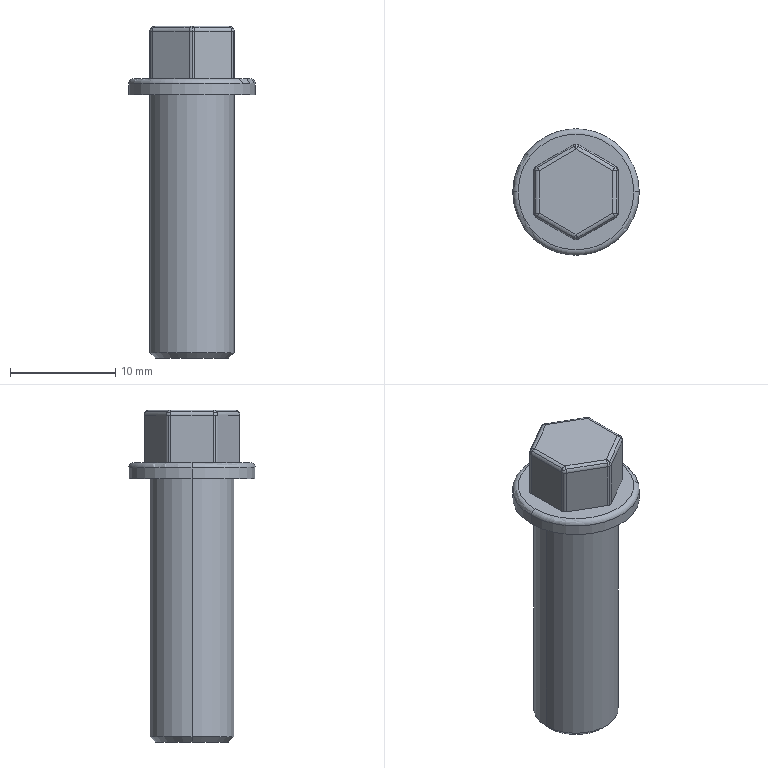Part | SolidWorks | features BaseBody 1 | 1 solid | 54 faces | box 12 x 12 x 31.5 mm | volume 1697 mm3 | cylinder 28 | sphere 12 | plane 10 | torus 2 | cone 2 | commonest cylinder face diameters 1 x24 8 x2 12 x2
STEP:
#1=CARTESIAN_POINT('',(-3.947,2.021,6.224));
#2=VERTEX_POINT('',#1);
#3=CARTESIAN_POINT('',(-4.,2.021,6.));
#4=VERTEX_POINT('',#3);
#5=CARTESIAN_POINT('',(-3.5,2.021,6.));
#6=DIRECTION('',(0.,-1.,0.));
#7=DIRECTION('',(0.,0.,1.));
#8=AXIS2_PLACEMENT_3D('',#5,#6,#7);
#9=CIRCLE('',#8,0.5);
#10=EDGE_CURVE('',#2,#4,#9,.T.);
#11=ORIENTED_EDGE('',*,*,#10,.F.);
#12=CARTESIAN_POINT('',(-3.724,2.408,6.224));
#13=VERTEX_POINT('',#12);
#14=CARTESIAN_POINT('',(-3.5,2.021,6.));
#15=DIRECTION('',(-0.433,0.25,-0.866));
#16=DIRECTION('',(-0.8944,0.,0.4472));
#17=AXIS2_PLACEMENT_3D('',#14,#15,#16);
#18=CIRCLE('',#17,0.5);
#19=EDGE_CURVE('',#2,#13,#18,.T.);
#20=ORIENTED_EDGE('',*,*,#19,.T.);
#21=CARTESIAN_POINT('',(-3.75,2.454,6.));
#22=VERTEX_POINT('',#21);
#23=CARTESIAN_POINT('',(-3.5,2.021,6.));
#24=DIRECTION('',(0.866,0.5,0.));
#25=DIRECTION('',(-0.5,0.866,0.));
#26=AXIS2_PLACEMENT_3D('',#23,#24,#25);
#27=CIRCLE('',#26,0.5);
#28=EDGE_CURVE('',#22,#13,#27,.T.);
#29=ORIENTED_EDGE('',*,*,#28,.F.);
#30=CARTESIAN_POINT('',(-3.933,2.271,6.));
#31=VERTEX_POINT('',#30);
#32=CARTESIAN_POINT('',(-3.5,2.021,6.));
#33=DIRECTION('',(0.,0.,-1.));
#34=DIRECTION('',(-1.,0.,0.));
#35=AXIS2_PLACEMENT_3D('',#32,#33,#34);
#36=CIRCLE('',#35,0.5);
#37=EDGE_CURVE('',#31,#22,#36,.T.);
#38=ORIENTED_EDGE('',*,*,#37,.F.);
#39=CARTESIAN_POINT('',(-3.5,2.021,6.));
#40=DIRECTION('',(0.,0.,-1.));
#41=DIRECTION('',(-1.,0.,0.));
#42=AXIS2_PLACEMENT_3D('',#39,#40,#41);
#43=CIRCLE('',#42,0.5);
#44=EDGE_CURVE('',#4,#31,#43,.T.);
#45=ORIENTED_EDGE('',*,*,#44,.F.);
#46=EDGE_LOOP('',(#11,#20,#29,#38,#45));
#47=FACE_OUTER_BOUND('',#46,.T.);
#48=CARTESIAN_POINT('',(-3.5,2.021,6.));
#49=DIRECTION('',(0.433,-0.25,0.866));
#50=DIRECTION('',(-0.75,0.433,0.5));
#51=AXIS2_PLACEMENT_3D('',#48,#49,#50);
#52=SPHERICAL_SURFACE('',#51,0.5);
#53=ADVANCED_FACE('',(#47),#52,.T.);
#54=ORIENTED_EDGE('',*,*,#44,.T.);
#55=CARTESIAN_POINT('',(-3.933,2.271,1.5));
#56=VERTEX_POINT('',#55);
#57=CARTESIAN_POINT('',(-3.933,2.271,1.5));
#58=DIRECTION('',(0.,0.,-1.));
#59=VECTOR('',#58,1000.);
#60=LINE('',#57,#59);
#61=EDGE_CURVE('',#31,#56,#60,.T.);
#62=ORIENTED_EDGE('',*,*,#61,.T.);
#63=CARTESIAN_POINT('',(-4.,2.021,1.5));
#64=VERTEX_POINT('',#63);
#65=CARTESIAN_POINT('',(-3.5,2.021,1.5));
#66=DIRECTION('',(0.,0.,1.));
#67=DIRECTION('',(-0.866,0.5,0.));
#68=AXIS2_PLACEMENT_3D('',#65,#66,#67);
#69=CIRCLE('',#68,0.5);
#70=EDGE_CURVE('',#56,#64,#69,.T.);
#71=ORIENTED_EDGE('',*,*,#70,.T.);
#72=CARTESIAN_POINT('',(-4.,2.021,1.5));
#73=DIRECTION('',(0.,0.,1.));
#74=VECTOR('',#73,1000.);
#75=LINE('',#72,#74);
#76=EDGE_CURVE('',#64,#4,#75,.T.);
#77=ORIENTED_EDGE('',*,*,#76,.T.);
#78=EDGE_LOOP('',(#54,#62,#71,#77));
#79=FACE_OUTER_BOUND('',#78,.T.);
#80=CARTESIAN_POINT('',(-3.5,2.021,1.5));
#81=DIRECTION('',(0.,0.,-1.));
#82=DIRECTION('',(-0.866,0.5,0.));
#83=AXIS2_PLACEMENT_3D('',#80,#81,#82);
#84=CYLINDRICAL_SURFACE('',#83,0.5);
#85=ADVANCED_FACE('',(#79),#84,.T.);
#86=CARTESIAN_POINT('',(-3.724,-2.408,6.224));
#87=VERTEX_POINT('',#86);
#88=CARTESIAN_POINT('',(-3.75,-2.454,6.));
#89=VERTEX_POINT('',#88);
#90=CARTESIAN_POINT('',(-3.5,-2.021,6.));
#91=DIRECTION('',(0.866,-0.5,0.));
#92=DIRECTION('',(0.,0.,1.));
#93=AXIS2_PLACEMENT_3D('',#90,#91,#92);
#94=CIRCLE('',#93,0.5);
#95=EDGE_CURVE('',#87,#89,#94,.T.);
#96=ORIENTED_EDGE('',*,*,#95,.F.);
#97=CARTESIAN_POINT('',(-3.947,-2.021,6.224));
#98=VERTEX_POINT('',#97);
#99=CARTESIAN_POINT('',(-3.5,-2.021,6.));
#100=DIRECTION('',(-0.433,-0.25,-0.866));
#101=DIRECTION('',(-0.8944,0.,0.4472));
#102=AXIS2_PLACEMENT_3D('',#99,#100,#101);
#103=CIRCLE('',#102,0.5);
#104=EDGE_CURVE('',#87,#98,#103,.T.);
#105=ORIENTED_EDGE('',*,*,#104,.T.);
#106=CARTESIAN_POINT('',(-4.,-2.021,6.));
#107=VERTEX_POINT('',#106);
#108=CARTESIAN_POINT('',(-3.5,-2.021,6.));
#109=DIRECTION('',(0.,1.,0.));
#110=DIRECTION('',(-1.,0.,0.));
#111=AXIS2_PLACEMENT_3D('',#108,#109,#110);
#112=CIRCLE('',#111,0.5);
#113=EDGE_CURVE('',#107,#98,#112,.T.);
#114=ORIENTED_EDGE('',*,*,#113,.F.);
#115=CARTESIAN_POINT('',(-3.933,-2.271,6.));
#116=VERTEX_POINT('',#115);
#117=CARTESIAN_POINT('',(-3.5,-2.021,6.));
#118=DIRECTION('',(0.,0.,-1.));
#119=DIRECTION('',(-0.5,-0.866,0.));
#120=AXIS2_PLACEMENT_3D('',#117,#118,#119);
#121=CIRCLE('',#120,0.5);
#122=EDGE_CURVE('',#116,#107,#121,.T.);
#123=ORIENTED_EDGE('',*,*,#122,.F.);
#124=CARTESIAN_POINT('',(-3.5,-2.021,6.));
#125=DIRECTION('',(0.,0.,-1.));
#126=DIRECTION('',(-0.5,-0.866,0.));
#127=AXIS2_PLACEMENT_3D('',#124,#125,#126);
#128=CIRCLE('',#127,0.5);
#129=EDGE_CURVE('',#89,#116,#128,.T.);
#130=ORIENTED_EDGE('',*,*,#129,.F.);
#131=EDGE_LOOP('',(#96,#105,#114,#123,#130));
#132=FACE_OUTER_BOUND('',#131,.T.);
#133=CARTESIAN_POINT('',(-3.5,-2.021,6.));
#134=DIRECTION('',(0.433,0.25,0.866));
#135=DIRECTION('',(-0.75,-0.433,0.5));
#136=AXIS2_PLACEMENT_3D('',#133,#134,#135);
#137=SPHERICAL_SURFACE('',#136,0.5);
#138=ADVANCED_FACE('',(#132),#137,.T.);
#139=ORIENTED_EDGE('',*,*,#129,.T.);
#140=CARTESIAN_POINT('',(-3.933,-2.271,1.5));
#141=VERTEX_POINT('',#140);
#142=CARTESIAN_POINT('',(-3.933,-2.271,1.5));
#143=DIRECTION('',(0.,0.,-1.));
#144=VECTOR('',#143,1000.);
#145=LINE('',#142,#144);
#146=EDGE_CURVE('',#116,#141,#145,.T.);
#147=ORIENTED_EDGE('',*,*,#146,.T.);
#148=CARTESIAN_POINT('',(-3.75,-2.454,1.5));
#149=VERTEX_POINT('',#148);
#150=CARTESIAN_POINT('',(-3.5,-2.021,1.5));
#151=DIRECTION('',(0.,0.,1.));
#152=DIRECTION('',(-0.866,-0.5,0.));
#153=AXIS2_PLACEMENT_3D('',#150,#151,#152);
#154=CIRCLE('',#153,0.5);
#155=EDGE_CURVE('',#141,#149,#154,.T.);
#156=ORIENTED_EDGE('',*,*,#155,.T.);
#157=CARTESIAN_POINT('',(-3.75,-2.454,1.5));
#158=DIRECTION('',(0.,0.,1.));
#159=VECTOR('',#158,1000.);
#160=LINE('',#157,#159);
#161=EDGE_CURVE('',#149,#89,#160,.T.);
#162=ORIENTED_EDGE('',*,*,#161,.T.);
#163=EDGE_LOOP('',(#139,#147,#156,#162));
#164=FACE_OUTER_BOUND('',#163,.T.);
#165=CARTESIAN_POINT('',(-3.5,-2.021,1.5));
#166=DIRECTION('',(0.,0.,-1.));
#167=DIRECTION('',(-0.866,-0.5,0.));
#168=AXIS2_PLACEMENT_3D('',#165,#166,#167);
#169=CYLINDRICAL_SURFACE('',#168,0.5);
#170=ADVANCED_FACE('',(#164),#169,.T.);
#171=CARTESIAN_POINT('',(0.,4.041,6.5));
#172=VERTEX_POINT('',#171);
#173=CARTESIAN_POINT('',(-0.1768,4.348,6.354));
#174=VERTEX_POINT('',#173);
#175=CARTESIAN_POINT('',(0.,4.041,6.));
#176=DIRECTION('',(-0.866,-0.5,0.));
#177=DIRECTION('',(0.,0.,1.));
#178=AXIS2_PLACEMENT_3D('',#175,#176,#177);
#179=CIRCLE('',#178,0.5);
#180=EDGE_CURVE('',#172,#174,#179,.T.);
#181=ORIENTED_EDGE('',*,*,#180,.F.);
#182=CARTESIAN_POINT('',(0.,4.541,6.));
#183=VERTEX_POINT('',#182);
#184=CARTESIAN_POINT('',(0.,4.041,6.));
#185=DIRECTION('',(-1.,0.,0.));
#186=DIRECTION('',(0.,-1.,0.));
#187=AXIS2_PLACEMENT_3D('',#184,#185,#186);
#188=CIRCLE('',#187,0.5);
#189=EDGE_CURVE('',#172,#183,#188,.T.);
#190=ORIENTED_EDGE('',*,*,#189,.T.);
#191=CARTESIAN_POINT('',(-0.25,4.474,6.));
#192=VERTEX_POINT('',#191);
#193=CARTESIAN_POINT('',(0.,4.041,6.));
#194=DIRECTION('',(0.,0.,-1.));
#195=DIRECTION('',(-0.5,0.866,0.));
#196=AXIS2_PLACEMENT_3D('',#193,#194,#195);
#197=CIRCLE('',#196,0.5);
#198=EDGE_CURVE('',#192,#183,#197,.T.);
#199=ORIENTED_EDGE('',*,*,#198,.F.);
#200=CARTESIAN_POINT('',(0.,4.041,6.));
#201=DIRECTION('',(-0.866,-0.5,0.));
#202=DIRECTION('',(0.,0.,1.));
#203=AXIS2_PLACEMENT_3D('',#200,#201,#202);
#204=CIRCLE('',#203,0.5);
#205=EDGE_CURVE('',#174,#192,#204,.T.);
#206=ORIENTED_EDGE('',*,*,#205,.F.);
#207=EDGE_LOOP('',(#181,#190,#199,#206));
#208=FACE_OUTER_BOUND('',#207,.T.);
#209=CARTESIAN_POINT('',(0.,4.041,6.));
#210=DIRECTION('',(1.,0.,0.));
#211=DIRECTION('',(0.,0.866,0.5));
#212=AXIS2_PLACEMENT_3D('',#209,#210,#211);
#213=SPHERICAL_SURFACE('',#212,0.5);
#214=ADVANCED_FACE('',(#208),#213,.T.);
#215=ORIENTED_EDGE('',*,*,#198,.T.);
#216=CARTESIAN_POINT('',(0.,4.541,1.5));
#217=VERTEX_POINT('',#216);
#218=CARTESIAN_POINT('',(0.,4.541,1.5));
#219=DIRECTION('',(0.,0.,-1.));
#220=VECTOR('',#219,1000.);
#221=LINE('',#218,#220);
#222=EDGE_CURVE('',#183,#217,#221,.T.);
#223=ORIENTED_EDGE('',*,*,#222,.T.);
#224=CARTESIAN_POINT('',(-0.25,4.474,1.5));
#225=VERTEX_POINT('',#224);
#226=CARTESIAN_POINT('',(0.,4.041,1.5));
#227=DIRECTION('',(0.,0.,1.));
#228=DIRECTION('',(0.,1.,0.));
#229=AXIS2_PLACEMENT_3D('',#226,#227,#228);
#230=CIRCLE('',#229,0.5);
#231=EDGE_CURVE('',#217,#225,#230,.T.);
#232=ORIENTED_EDGE('',*,*,#231,.T.);
#233=CARTESIAN_POINT('',(-0.25,4.474,1.5));
#234=DIRECTION('',(0.,0.,1.));
#235=VECTOR('',#234,1000.);
#236=LINE('',#233,#235);
#237=EDGE_CURVE('',#225,#192,#236,.T.);
#238=ORIENTED_EDGE('',*,*,#237,.T.);
#239=EDGE_LOOP('',(#215,#223,#232,#238));
#240=FACE_OUTER_BOUND('',#239,.T.);
#241=CARTESIAN_POINT('',(0.,4.041,1.5));
#242=DIRECTION('',(0.,0.,-1.));
#243=DIRECTION('',(0.,1.,0.));
#244=AXIS2_PLACEMENT_3D('',#241,#242,#243);
#245=CYLINDRICAL_SURFACE('',#244,0.5);
#246=ADVANCED_FACE('',(#240),#245,.T.);
#247=ORIENTED_EDGE('',*,*,#28,.T.);
#248=CARTESIAN_POINT('',(-3.677,2.327,6.354));
#249=VERTEX_POINT('',#248);
#250=CARTESIAN_POINT('',(-3.5,2.021,6.));
#251=DIRECTION('',(0.866,0.5,0.));
#252=DIRECTION('',(-0.5,0.866,0.));
#253=AXIS2_PLACEMENT_3D('',#250,#251,#252);
#254=CIRCLE('',#253,0.5);
#255=EDGE_CURVE('',#13,#249,#254,.T.);
#256=ORIENTED_EDGE('',*,*,#255,.T.);
#257=CARTESIAN_POINT('',(-0.9268,3.915,6.354));
#258=DIRECTION('',(0.866,0.5,0.));
#259=VECTOR('',#258,1000.);
#260=LINE('',#257,#259);
#261=EDGE_CURVE('',#249,#174,#260,.T.);
#262=ORIENTED_EDGE('',*,*,#261,.T.);
#263=ORIENTED_EDGE('',*,*,#205,.T.);
#264=CARTESIAN_POINT('',(-1.,4.041,6.));
#265=DIRECTION('',(-0.866,-0.5,0.));
#266=VECTOR('',#265,1000.);
#267=LINE('',#264,#266);
#268=EDGE_CURVE('',#192,#22,#267,.T.);
#269=ORIENTED_EDGE('',*,*,#268,.T.);
#270=EDGE_LOOP('',(#247,#256,#262,#263,#269));
#271=FACE_OUTER_BOUND('',#270,.T.);
#272=CARTESIAN_POINT('',(-0.75,3.608,6.));
#273=DIRECTION('',(0.866,0.5,0.));
#274=DIRECTION('',(-0.3536,0.6124,0.7071));
#275=AXIS2_PLACEMENT_3D('',#272,#273,#274);
#276=CYLINDRICAL_SURFACE('',#275,0.5);
#277=ADVANCED_FACE('',(#271),#276,.T.);
#278=CARTESIAN_POINT('',(0.,-4.541,6.));
#279=VERTEX_POINT('',#278);
#280=CARTESIAN_POINT('',(-0.25,-4.474,6.));
#281=VERTEX_POINT('',#280);
#282=CARTESIAN_POINT('',(0.,-4.041,6.));
#283=DIRECTION('',(0.,0.,-1.));
#284=DIRECTION('',(0.5,-0.866,0.));
#285=AXIS2_PLACEMENT_3D('',#282,#283,#284);
#286=CIRCLE('',#285,0.5);
#287=EDGE_CURVE('',#279,#281,#286,.T.);
#288=ORIENTED_EDGE('',*,*,#287,.F.);
#289=CARTESIAN_POINT('',(0.,-4.041,6.5));
#290=VERTEX_POINT('',#289);
#291=CARTESIAN_POINT('',(0.,-4.041,6.));
#292=DIRECTION('',(-1.,0.,0.));
#293=DIRECTION('',(0.,-1.,0.));
#294=AXIS2_PLACEMENT_3D('',#291,#292,#293);
#295=CIRCLE('',#294,0.5);
#296=EDGE_CURVE('',#279,#290,#295,.T.);
#297=ORIENTED_EDGE('',*,*,#296,.T.);
#298=CARTESIAN_POINT('',(-0.1768,-4.348,6.354));
#299=VERTEX_POINT('',#298);
#300=CARTESIAN_POINT('',(0.,-4.041,6.));
#301=DIRECTION('',(-0.866,0.5,0.));
#302=DIRECTION('',(-0.5,-0.866,0.));
#303=AXIS2_PLACEMENT_3D('',#300,#301,#302);
#304=CIRCLE('',#303,0.5);
#305=EDGE_CURVE('',#299,#290,#304,.T.);
#306=ORIENTED_EDGE('',*,*,#305,.F.);
#307=CARTESIAN_POINT('',(0.,-4.041,6.));
#308=DIRECTION('',(-0.866,0.5,0.));
#309=DIRECTION('',(-0.5,-0.866,0.));
#310=AXIS2_PLACEMENT_3D('',#307,#308,#309);
#311=CIRCLE('',#310,0.5);
#312=EDGE_CURVE('',#281,#299,#311,.T.);
#313=ORIENTED_EDGE('',*,*,#312,.F.);
#314=EDGE_LOOP('',(#288,#297,#306,#313));
#315=FACE_OUTER_BOUND('',#314,.T.);
#316=CARTESIAN_POINT('',(0.,-4.041,6.));
#317=DIRECTION('',(1.,0.,0.));
#318=DIRECTION('',(0.,-0.866,0.5));
#319=AXIS2_PLACEMENT_3D('',#316,#317,#318);
#320=SPHERICAL_SURFACE('',#319,0.5);
#321=ADVANCED_FACE('',(#315),#320,.T.);
#322=CARTESIAN_POINT('',(0.25,-4.474,6.));
#323=VERTEX_POINT('',#322);
#324=CARTESIAN_POINT('',(0.,-4.041,6.));
#325=DIRECTION('',(0.,0.,-1.));
#326=DIRECTION('',(0.5,-0.866,0.));
#327=AXIS2_PLACEMENT_3D('',#324,#325,#326);
#328=CIRCLE('',#327,0.5);
#329=EDGE_CURVE('',#323,#279,#328,.T.);
#330=ORIENTED_EDGE('',*,*,#329,.T.);
#331=CARTESIAN_POINT('',(0.,-4.541,1.5));
#332=VERTEX_POINT('',#331);
#333=CARTESIAN_POINT('',(0.,-4.541,1.5));
#334=DIRECTION('',(0.,0.,-1.));
#335=VECTOR('',#334,1000.);
#336=LINE('',#333,#335);
#337=EDGE_CURVE('',#279,#332,#336,.T.);
#338=ORIENTED_EDGE('',*,*,#337,.T.);
#339=CARTESIAN_POINT('',(0.25,-4.474,1.5));
#340=VERTEX_POINT('',#339);
#341=CARTESIAN_POINT('',(0.,-4.041,1.5));
#342=DIRECTION('',(0.,0.,1.));
#343=DIRECTION('',(0.,-1.,0.));
#344=AXIS2_PLACEMENT_3D('',#341,#342,#343);
#345=CIRCLE('',#344,0.5);
#346=EDGE_CURVE('',#332,#340,#345,.T.);
#347=ORIENTED_EDGE('',*,*,#346,.T.);
#348=CARTESIAN_POINT('',(0.25,-4.474,1.5));
#349=DIRECTION('',(0.,0.,1.));
#350=VECTOR('',#349,1000.);
#351=LINE('',#348,#350);
#352=EDGE_CURVE('',#340,#323,#351,.T.);
#353=ORIENTED_EDGE('',*,*,#352,.T.);
#354=EDGE_LOOP('',(#330,#338,#347,#353));
#355=FACE_OUTER_BOUND('',#354,.T.);
#356=CARTESIAN_POINT('',(0.,-4.041,1.5));
#357=DIRECTION('',(0.,0.,-1.));
#358=DIRECTION('',(0.,-1.,0.));
#359=AXIS2_PLACEMENT_3D('',#356,#357,#358);
#360=CYLINDRICAL_SURFACE('',#359,0.5);
#361=ADVANCED_FACE('',(#355),#360,.T.);
#362=CARTESIAN_POINT('',(3.724,2.408,6.224));
#363=VERTEX_POINT('',#362);
#364=CARTESIAN_POINT('',(3.75,2.454,6.));
#365=VERTEX_POINT('',#364);
#366=CARTESIAN_POINT('',(3.5,2.021,6.));
#367=DIRECTION('',(-0.866,0.5,0.));
#368=DIRECTION('',(0.,0.,1.));
#369=AXIS2_PLACEMENT_3D('',#366,#367,#368);
#370=CIRCLE('',#369,0.5);
#371=EDGE_CURVE('',#363,#365,#370,.T.);
#372=ORIENTED_EDGE('',*,*,#371,.F.);
#373=CARTESIAN_POINT('',(3.947,2.021,6.224));
#374=VERTEX_POINT('',#373);
#375=CARTESIAN_POINT('',(3.5,2.021,6.));
#376=DIRECTION('',(0.433,0.25,-0.866));
#377=DIRECTION('',(-0.8944,0.,-0.4472));
#378=AXIS2_PLACEMENT_3D('',#375,#376,#377);
#379=CIRCLE('',#378,0.5);
#380=EDGE_CURVE('',#363,#374,#379,.T.);
#381=ORIENTED_EDGE('',*,*,#380,.T.);
#382=CARTESIAN_POINT('',(4.,2.021,6.));
#383=VERTEX_POINT('',#382);
#384=CARTESIAN_POINT('',(3.5,2.021,6.));
#385=DIRECTION('',(0.,-1.,0.));
#386=DIRECTION('',(1.,0.,0.));
#387=AXIS2_PLACEMENT_3D('',#384,#385,#386);
#388=CIRCLE('',#387,0.5);
#389=EDGE_CURVE('',#383,#374,#388,.T.);
#390=ORIENTED_EDGE('',*,*,#389,.F.);
#391=CARTESIAN_POINT('',(3.933,2.271,6.));
#392=VERTEX_POINT('',#391);
#393=CARTESIAN_POINT('',(3.5,2.021,6.));
#394=DIRECTION('',(0.,0.,-1.));
#395=DIRECTION('',(0.5,0.866,0.));
#396=AXIS2_PLACEMENT_3D('',#393,#394,#395);
#397=CIRCLE('',#396,0.5);
#398=EDGE_CURVE('',#392,#383,#397,.T.);
#399=ORIENTED_EDGE('',*,*,#398,.F.);
#400=CARTESIAN_POINT('',(3.5,2.021,6.));
#401=DIRECTION('',(0.,0.,-1.));
#402=DIRECTION('',(0.5,0.866,0.));
#403=AXIS2_PLACEMENT_3D('',#400,#401,#402);
#404=CIRCLE('',#403,0.5);
#405=EDGE_CURVE('',#365,#392,#404,.T.);
#406=ORIENTED_EDGE('',*,*,#405,.F.);
#407=EDGE_LOOP('',(#372,#381,#390,#399,#406));
#408=FACE_OUTER_BOUND('',#407,.T.);
#409=CARTESIAN_POINT('',(3.5,2.021,6.));
#410=DIRECTION('',(-0.433,-0.25,0.866));
#411=DIRECTION('',(0.75,0.433,0.5));
#412=AXIS2_PLACEMENT_3D('',#409,#410,#411);
#413=SPHERICAL_SURFACE('',#412,0.5);
#414=ADVANCED_FACE('',(#408),#413,.T.);
#415=ORIENTED_EDGE('',*,*,#405,.T.);
#416=CARTESIAN_POINT('',(3.933,2.271,1.5));
#417=VERTEX_POINT('',#416);
#418=CARTESIAN_POINT('',(3.933,2.271,1.5));
#419=DIRECTION('',(0.,0.,-1.));
#420=VECTOR('',#419,1000.);
#421=LINE('',#418,#420);
#422=EDGE_CURVE('',#392,#417,#421,.T.);
#423=ORIENTED_EDGE('',*,*,#422,.T.);
#424=CARTESIAN_POINT('',(3.75,2.454,1.5));
#425=VERTEX_POINT('',#424);
#426=CARTESIAN_POINT('',(3.5,2.021,1.5));
#427=DIRECTION('',(0.,0.,1.));
#428=DIRECTION('',(0.866,0.5,0.));
#429=AXIS2_PLACEMENT_3D('',#426,#427,#428);
#430=CIRCLE('',#429,0.5);
#431=EDGE_CURVE('',#417,#425,#430,.T.);
#432=ORIENTED_EDGE('',*,*,#431,.T.);
#433=CARTESIAN_POINT('',(3.75,2.454,1.5));
#434=DIRECTION('',(0.,0.,1.));
#435=VECTOR('',#434,1000.);
#436=LINE('',#433,#435);
#437=EDGE_CURVE('',#425,#365,#436,.T.);
#438=ORIENTED_EDGE('',*,*,#437,.T.);
#439=EDGE_LOOP('',(#415,#423,#432,#438));
#440=FACE_OUTER_BOUND('',#439,.T.);
#441=CARTESIAN_POINT('',(3.5,2.021,1.5));
#442=DIRECTION('',(0.,0.,-1.));
#443=DIRECTION('',(0.866,0.5,0.));
#444=AXIS2_PLACEMENT_3D('',#441,#442,#443);
#445=CYLINDRICAL_SURFACE('',#444,0.5);
#446=ADVANCED_FACE('',(#440),#445,.T.);
#447=CARTESIAN_POINT('',(0.25,4.474,6.));
#448=VERTEX_POINT('',#447);
#449=CARTESIAN_POINT('',(0.1768,4.348,6.354));
#450=VERTEX_POINT('',#449);
#451=CARTESIAN_POINT('',(0.,4.041,6.));
#452=DIRECTION('',(0.866,-0.5,0.));
#453=DIRECTION('',(0.5,0.866,0.));
#454=AXIS2_PLACEMENT_3D('',#451,#452,#453);
#455=CIRCLE('',#454,0.5);
#456=EDGE_CURVE('',#448,#450,#455,.T.);
#457=ORIENTED_EDGE('',*,*,#456,.T.);
#458=CARTESIAN_POINT('',(3.677,2.327,6.354));
#459=VERTEX_POINT('',#458);
#460=CARTESIAN_POINT('',(2.927,2.76,6.354));
#461=DIRECTION('',(0.866,-0.5,0.));
#462=VECTOR('',#461,1000.);
#463=LINE('',#460,#462);
#464=EDGE_CURVE('',#450,#459,#463,.T.);
#465=ORIENTED_EDGE('',*,*,#464,.T.);
#466=CARTESIAN_POINT('',(3.5,2.021,6.));
#467=DIRECTION('',(-0.866,0.5,0.));
#468=DIRECTION('',(0.,0.,1.));
#469=AXIS2_PLACEMENT_3D('',#466,#467,#468);
#470=CIRCLE('',#469,0.5);
#471=EDGE_CURVE('',#459,#363,#470,.T.);
#472=ORIENTED_EDGE('',*,*,#471,.T.);
#473=ORIENTED_EDGE('',*,*,#371,.T.);
#474=CARTESIAN_POINT('',(3.,2.887,6.));
#475=DIRECTION('',(-0.866,0.5,0.));
#476=VECTOR('',#475,1000.);
#477=LINE('',#474,#476);
#478=EDGE_CURVE('',#365,#448,#477,.T.);
#479=ORIENTED_EDGE('',*,*,#478,.T.);
#480=EDGE_LOOP('',(#457,#465,#472,#473,#479));
#481=FACE_OUTER_BOUND('',#480,.T.);
#482=CARTESIAN_POINT('',(2.75,2.454,6.));
#483=DIRECTION('',(0.866,-0.5,0.));
#484=DIRECTION('',(0.3536,0.6124,0.7071));
#485=AXIS2_PLACEMENT_3D('',#482,#483,#484);
#486=CYLINDRICAL_SURFACE('',#485,0.5);
#487=ADVANCED_FACE('',(#481),#486,.T.);
#488=CARTESIAN_POINT('',(3.947,-2.021,6.224));
#489=VERTEX_POINT('',#488);
#490=CARTESIAN_POINT('',(4.,-2.021,6.));
#491=VERTEX_POINT('',#490);
#492=CARTESIAN_POINT('',(3.5,-2.021,6.));
#493=DIRECTION('',(0.,1.,0.));
#494=DIRECTION('',(0.,0.,1.));
#495=AXIS2_PLACEMENT_3D('',#492,#493,#494);
#496=CIRCLE('',#495,0.5);
#497=EDGE_CURVE('',#489,#491,#496,.T.);
#498=ORIENTED_EDGE('',*,*,#497,.F.);
#499=CARTESIAN_POINT('',(3.724,-2.408,6.224));
#500=VERTEX_POINT('',#499);
#501=CARTESIAN_POINT('',(3.5,-2.021,6.));
#502=DIRECTION('',(0.433,-0.25,-0.866));
#503=DIRECTION('',(-0.8944,0.,-0.4472));
#504=AXIS2_PLACEMENT_3D('',#501,#502,#503);
#505=CIRCLE('',#504,0.5);
#506=EDGE_CURVE('',#489,#500,#505,.T.);
#507=ORIENTED_EDGE('',*,*,#506,.T.);
#508=CARTESIAN_POINT('',(3.75,-2.454,6.));
#509=VERTEX_POINT('',#508);
#510=CARTESIAN_POINT('',(3.5,-2.021,6.));
#511=DIRECTION('',(-0.866,-0.5,0.));
#512=DIRECTION('',(0.5,-0.866,0.));
#513=AXIS2_PLACEMENT_3D('',#510,#511,#512);
#514=CIRCLE('',#513,0.5);
#515=EDGE_CURVE('',#509,#500,#514,.T.);
#516=ORIENTED_EDGE('',*,*,#515,.F.);
#517=CARTESIAN_POINT('',(3.933,-2.271,6.));
#518=VERTEX_POINT('',#517);
#519=CARTESIAN_POINT('',(3.5,-2.021,6.));
#520=DIRECTION('',(0.,0.,-1.));
#521=DIRECTION('',(1.,0.,0.));
#522=AXIS2_PLACEMENT_3D('',#519,#520,#521);
#523=CIRCLE('',#522,0.5);
#524=EDGE_CURVE('',#518,#509,#523,.T.);
#525=ORIENTED_EDGE('',*,*,#524,.F.);
#526=CARTESIAN_POINT('',(3.5,-2.021,6.));
#527=DIRECTION('',(0.,0.,-1.));
#528=DIRECTION('',(1.,0.,0.));
#529=AXIS2_PLACEMENT_3D('',#526,#527,#528);
#530=CIRCLE('',#529,0.5);
#531=EDGE_CURVE('',#491,#518,#530,.T.);
#532=ORIENTED_EDGE('',*,*,#531,.F.);
#533=EDGE_LOOP('',(#498,#507,#516,#525,#532));
#534=FACE_OUTER_BOUND('',#533,.T.);
#535=CARTESIAN_POINT('',(3.5,-2.021,6.));
#536=DIRECTION('',(-0.433,0.25,0.866));
#537=DIRECTION('',(0.75,-0.433,0.5));
#538=AXIS2_PLACEMENT_3D('',#535,#536,#537);
#539=SPHERICAL_SURFACE('',#538,0.5);
#540=ADVANCED_FACE('',(#534),#539,.T.);
#541=ORIENTED_EDGE('',*,*,#531,.T.);
#542=CARTESIAN_POINT('',(3.933,-2.271,1.5));
#543=VERTEX_POINT('',#542);
#544=CARTESIAN_POINT('',(3.933,-2.271,1.5));
#545=DIRECTION('',(0.,0.,-1.));
#546=VECTOR('',#545,1000.);
#547=LINE('',#544,#546);
#548=EDGE_CURVE('',#518,#543,#547,.T.);
#549=ORIENTED_EDGE('',*,*,#548,.T.);
#550=CARTESIAN_POINT('',(4.,-2.021,1.5));
#551=VERTEX_POINT('',#550);
#552=CARTESIAN_POINT('',(3.5,-2.021,1.5));
#553=DIRECTION('',(0.,0.,1.));
#554=DIRECTION('',(0.866,-0.5,0.));
#555=AXIS2_PLACEMENT_3D('',#552,#553,#554);
#556=CIRCLE('',#555,0.5);
#557=EDGE_CURVE('',#543,#551,#556,.T.);
#558=ORIENTED_EDGE('',*,*,#557,.T.);
#559=CARTESIAN_POINT('',(4.,-2.021,1.5));
#560=DIRECTION('',(0.,0.,1.));
#561=VECTOR('',#560,1000.);
#562=LINE('',#559,#561);
#563=EDGE_CURVE('',#551,#491,#562,.T.);
#564=ORIENTED_EDGE('',*,*,#563,.T.);
#565=EDGE_LOOP('',(#541,#549,#558,#564));
#566=FACE_OUTER_BOUND('',#565,.T.);
#567=CARTESIAN_POINT('',(3.5,-2.021,1.5));
#568=DIRECTION('',(0.,0.,-1.));
#569=DIRECTION('',(0.866,-0.5,0.));
#570=AXIS2_PLACEMENT_3D('',#567,#568,#569);
#571=CYLINDRICAL_SURFACE('',#570,0.5);
#572=ADVANCED_FACE('',(#566),#571,.T.);
#573=ORIENTED_EDGE('',*,*,#389,.T.);
#574=CARTESIAN_POINT('',(3.854,2.021,6.354));
#575=VERTEX_POINT('',#574);
#576=CARTESIAN_POINT('',(3.5,2.021,6.));
#577=DIRECTION('',(0.,-1.,0.));
#578=DIRECTION('',(1.,0.,0.));
#579=AXIS2_PLACEMENT_3D('',#576,#577,#578);
#580=CIRCLE('',#579,0.5);
#581=EDGE_CURVE('',#374,#575,#580,.T.);
#582=ORIENTED_EDGE('',*,*,#581,.T.);
#583=CARTESIAN_POINT('',(3.854,-2.021,6.354));
#584=VERTEX_POINT('',#583);
#585=CARTESIAN_POINT('',(3.854,-1.155,6.354));
#586=DIRECTION('',(0.,-1.,0.));
#587=VECTOR('',#586,1000.);
#588=LINE('',#585,#587);
#589=EDGE_CURVE('',#575,#584,#588,.T.);
#590=ORIENTED_EDGE('',*,*,#589,.T.);
#591=CARTESIAN_POINT('',(3.5,-2.021,6.));
#592=DIRECTION('',(0.,1.,0.));
#593=DIRECTION('',(0.,0.,1.));
#594=AXIS2_PLACEMENT_3D('',#591,#592,#593);
#595=CIRCLE('',#594,0.5);
#596=EDGE_CURVE('',#584,#489,#595,.T.);
#597=ORIENTED_EDGE('',*,*,#596,.T.);
#598=ORIENTED_EDGE('',*,*,#497,.T.);
#599=CARTESIAN_POINT('',(4.,-1.155,6.));
#600=DIRECTION('',(0.,1.,0.));
#601=VECTOR('',#600,1000.);
#602=LINE('',#599,#601);
#603=EDGE_CURVE('',#491,#383,#602,.T.);
#604=ORIENTED_EDGE('',*,*,#603,.T.);
#605=EDGE_LOOP('',(#573,#582,#590,#597,#598,#604));
#606=FACE_OUTER_BOUND('',#605,.T.);
#607=CARTESIAN_POINT('',(3.5,-1.155,6.));
#608=DIRECTION('',(0.,-1.,0.));
#609=DIRECTION('',(0.7071,0.,0.7071));
#610=AXIS2_PLACEMENT_3D('',#607,#608,#609);
#611=CYLINDRICAL_SURFACE('',#610,0.5);
#612=ADVANCED_FACE('',(#606),#611,.T.);
#613=ORIENTED_EDGE('',*,*,#515,.T.);
#614=CARTESIAN_POINT('',(3.677,-2.327,6.354));
#615=VERTEX_POINT('',#614);
#616=CARTESIAN_POINT('',(3.5,-2.021,6.));
#617=DIRECTION('',(-0.866,-0.5,0.));
#618=DIRECTION('',(0.5,-0.866,0.));
#619=AXIS2_PLACEMENT_3D('',#616,#617,#618);
#620=CIRCLE('',#619,0.5);
#621=EDGE_CURVE('',#500,#615,#620,.T.);
#622=ORIENTED_EDGE('',*,*,#621,.T.);
#623=CARTESIAN_POINT('',(0.1768,-4.348,6.354));
#624=VERTEX_POINT('',#623);
#625=CARTESIAN_POINT('',(0.9268,-3.915,6.354));
#626=DIRECTION('',(-0.866,-0.5,0.));
#627=VECTOR('',#626,1000.);
#628=LINE('',#625,#627);
#629=EDGE_CURVE('',#615,#624,#628,.T.);
#630=ORIENTED_EDGE('',*,*,#629,.T.);
#631=CARTESIAN_POINT('',(0.,-4.041,6.));
#632=DIRECTION('',(0.866,0.5,0.));
#633=DIRECTION('',(0.,0.,1.));
#634=AXIS2_PLACEMENT_3D('',#631,#632,#633);
#635=CIRCLE('',#634,0.5);
#636=EDGE_CURVE('',#624,#323,#635,.T.);
#637=ORIENTED_EDGE('',*,*,#636,.T.);
#638=CARTESIAN_POINT('',(1.,-4.041,6.));
#639=DIRECTION('',(0.866,0.5,0.));
#640=VECTOR('',#639,1000.);
#641=LINE('',#638,#640);
#642=EDGE_CURVE('',#323,#509,#641,.T.);
#643=ORIENTED_EDGE('',*,*,#642,.T.);
#644=EDGE_LOOP('',(#613,#622,#630,#637,#643));
#645=FACE_OUTER_BOUND('',#644,.T.);
#646=CARTESIAN_POINT('',(0.75,-3.608,6.));
#647=DIRECTION('',(-0.866,-0.5,0.));
#648=DIRECTION('',(0.3536,-0.6124,0.7071));
#649=AXIS2_PLACEMENT_3D('',#646,#647,#648);
#650=CYLINDRICAL_SURFACE('',#649,0.5);
#651=ADVANCED_FACE('',(#645),#650,.T.);
#652=ORIENTED_EDGE('',*,*,#312,.T.);
#653=CARTESIAN_POINT('',(-3.677,-2.327,6.354));
#654=VERTEX_POINT('',#653);
#655=CARTESIAN_POINT('',(-2.927,-2.76,6.354));
#656=DIRECTION('',(-0.866,0.5,0.));
#657=VECTOR('',#656,1000.);
#658=LINE('',#655,#657);
#659=EDGE_CURVE('',#299,#654,#658,.T.);
#660=ORIENTED_EDGE('',*,*,#659,.T.);
#661=CARTESIAN_POINT('',(-3.5,-2.021,6.));
#662=DIRECTION('',(0.866,-0.5,0.));
#663=DIRECTION('',(0.,0.,1.));
#664=AXIS2_PLACEMENT_3D('',#661,#662,#663);
#665=CIRCLE('',#664,0.5);
#666=EDGE_CURVE('',#654,#87,#665,.T.);
#667=ORIENTED_EDGE('',*,*,#666,.T.);
#668=ORIENTED_EDGE('',*,*,#95,.T.);
#669=CARTESIAN_POINT('',(-3.,-2.887,6.));
#670=DIRECTION('',(0.866,-0.5,0.));
#671=VECTOR('',#670,1000.);
#672=LINE('',#669,#671);
#673=EDGE_CURVE('',#89,#281,#672,.T.);
#674=ORIENTED_EDGE('',*,*,#673,.T.);
#675=EDGE_LOOP('',(#652,#660,#667,#668,#674));
#676=FACE_OUTER_BOUND('',#675,.T.);
#677=CARTESIAN_POINT('',(-2.75,-2.454,6.));
#678=DIRECTION('',(-0.866,0.5,0.));
#679=DIRECTION('',(-0.3536,-0.6124,0.7071));
#680=AXIS2_PLACEMENT_3D('',#677,#678,#679);
#681=CYLINDRICAL_SURFACE('',#680,0.5);
#682=ADVANCED_FACE('',(#676),#681,.T.);
#683=ORIENTED_EDGE('',*,*,#113,.T.);
#684=CARTESIAN_POINT('',(-3.854,-2.021,6.354));
#685=VERTEX_POINT('',#684);
#686=CARTESIAN_POINT('',(-3.5,-2.021,6.));
#687=DIRECTION('',(0.,1.,0.));
#688=DIRECTION('',(-1.,0.,0.));
#689=AXIS2_PLACEMENT_3D('',#686,#687,#688);
#690=CIRCLE('',#689,0.5);
#691=EDGE_CURVE('',#98,#685,#690,.T.);
#692=ORIENTED_EDGE('',*,*,#691,.T.);
#693=CARTESIAN_POINT('',(-3.854,2.021,6.354));
#694=VERTEX_POINT('',#693);
#695=CARTESIAN_POINT('',(-3.854,1.155,6.354));
#696=DIRECTION('',(0.,1.,0.));
#697=VECTOR('',#696,1000.);
#698=LINE('',#695,#697);
#699=EDGE_CURVE('',#685,#694,#698,.T.);
#700=ORIENTED_EDGE('',*,*,#699,.T.);
#701=CARTESIAN_POINT('',(-3.5,2.021,6.));
#702=DIRECTION('',(0.,-1.,0.));
#703=DIRECTION('',(0.,0.,1.));
#704=AXIS2_PLACEMENT_3D('',#701,#702,#703);
#705=CIRCLE('',#704,0.5);
#706=EDGE_CURVE('',#694,#2,#705,.T.);
#707=ORIENTED_EDGE('',*,*,#706,.T.);
#708=ORIENTED_EDGE('',*,*,#10,.T.);
#709=CARTESIAN_POINT('',(-4.,1.155,6.));
#710=DIRECTION('',(0.,-1.,0.));
#711=VECTOR('',#710,1000.);
#712=LINE('',#709,#711);
#713=EDGE_CURVE('',#4,#107,#712,.T.);
#714=ORIENTED_EDGE('',*,*,#713,.T.);
#715=EDGE_LOOP('',(#683,#692,#700,#707,#708,#714));
#716=FACE_OUTER_BOUND('',#715,.T.);
#717=CARTESIAN_POINT('',(-3.5,1.155,6.));
#718=DIRECTION('',(0.,1.,0.));
#719=DIRECTION('',(-0.7071,0.,0.7071));
#720=AXIS2_PLACEMENT_3D('',#717,#718,#719);
#721=CYLINDRICAL_SURFACE('',#720,0.5);
#722=ADVANCED_FACE('',(#716),#721,.T.);
#723=CARTESIAN_POINT('',(6.,0.,1.));
#724=VERTEX_POINT('',#723);
#725=CARTESIAN_POINT('',(-6.,0.,1.));
#726=VERTEX_POINT('',#725);
#727=CARTESIAN_POINT('',(0.,0.,1.));
#728=DIRECTION('',(0.,0.,1.));
#729=DIRECTION('',(-1.,0.,0.));
#730=AXIS2_PLACEMENT_3D('',#727,#728,#729);
#731=CIRCLE('',#730,6.);
#732=EDGE_CURVE('',#724,#726,#731,.T.);
#733=ORIENTED_EDGE('',*,*,#732,.T.);
#734=CARTESIAN_POINT('',(-5.5,0.,1.5));
#735=VERTEX_POINT('',#734);
#736=CARTESIAN_POINT('',(-5.5,0.,1.));
#737=DIRECTION('',(0.,1.,0.));
#738=DIRECTION('',(-1.,0.,0.));
#739=AXIS2_PLACEMENT_3D('',#736,#737,#738);
#740=CIRCLE('',#739,0.5);
#741=EDGE_CURVE('',#726,#735,#740,.T.);
#742=ORIENTED_EDGE('',*,*,#741,.T.);
#743=CARTESIAN_POINT('',(5.5,0.,1.5));
#744=VERTEX_POINT('',#743);
#745=CARTESIAN_POINT('',(0.,0.,1.5));
#746=DIRECTION('',(0.,0.,-1.));
#747=DIRECTION('',(-1.,0.,0.));
#748=AXIS2_PLACEMENT_3D('',#745,#746,#747);
#749=CIRCLE('',#748,5.5);
#750=EDGE_CURVE('',#735,#744,#749,.T.);
#751=ORIENTED_EDGE('',*,*,#750,.T.);
#752=CARTESIAN_POINT('',(5.5,0.,1.));
#753=DIRECTION('',(0.,-1.,0.));
#754=DIRECTION('',(0.,0.,-1.));
#755=AXIS2_PLACEMENT_3D('',#752,#753,#754);
#756=CIRCLE('',#755,0.5);
#757=EDGE_CURVE('',#724,#744,#756,.T.);
#758=ORIENTED_EDGE('',*,*,#757,.F.);
#759=EDGE_LOOP('',(#733,#742,#751,#758));
#760=FACE_OUTER_BOUND('',#759,.T.);
#761=CARTESIAN_POINT('',(0.,0.,1.));
#762=DIRECTION('',(0.,0.,1.));
#763=DIRECTION('',(1.,0.,0.));
#764=AXIS2_PLACEMENT_3D('',#761,#762,#763);
#765=TOROIDAL_SURFACE('',#764,5.5,0.5);
#766=ADVANCED_FACE('',(#760),#765,.T.);
#767=ORIENTED_EDGE('',*,*,#732,.F.);
#768=CARTESIAN_POINT('',(6.,0.,0.));
#769=VERTEX_POINT('',#768);
#770=CARTESIAN_POINT('',(6.,0.,0.));
#771=DIRECTION('',(0.,0.,-1.));
#772=VECTOR('',#771,1000.);
#773=LINE('',#770,#772);
#774=EDGE_CURVE('',#724,#769,#773,.T.);
#775=ORIENTED_EDGE('',*,*,#774,.T.);
#776=CARTESIAN_POINT('',(-6.,0.,0.));
#777=VERTEX_POINT('',#776);
#778=CARTESIAN_POINT('',(0.,0.,0.));
#779=DIRECTION('',(0.,0.,-1.));
#780=DIRECTION('',(-1.,0.,0.));
#781=AXIS2_PLACEMENT_3D('',#778,#779,#780);
#782=CIRCLE('',#781,6.);
#783=EDGE_CURVE('',#777,#769,#782,.T.);
#784=ORIENTED_EDGE('',*,*,#783,.F.);
#785=CARTESIAN_POINT('',(-6.,0.,0.));
#786=DIRECTION('',(0.,0.,-1.));
#787=VECTOR('',#786,1000.);
#788=LINE('',#785,#787);
#789=EDGE_CURVE('',#726,#777,#788,.T.);
#790=ORIENTED_EDGE('',*,*,#789,.F.);
#791=EDGE_LOOP('',(#767,#775,#784,#790));
#792=FACE_OUTER_BOUND('',#791,.T.);
#793=CARTESIAN_POINT('',(0.,0.,0.));
#794=DIRECTION('',(0.,0.,-1.));
#795=DIRECTION('',(-1.,0.,0.));
#796=AXIS2_PLACEMENT_3D('',#793,#794,#795);
#797=CYLINDRICAL_SURFACE('',#796,6.);
#798=ADVANCED_FACE('',(#792),#797,.T.);
#799=CARTESIAN_POINT('',(3.5,0.,-25.));
#800=VERTEX_POINT('',#799);
#801=CARTESIAN_POINT('',(-3.5,0.,-25.));
#802=VERTEX_POINT('',#801);
#803=CARTESIAN_POINT('',(0.,0.,-25.));
#804=DIRECTION('',(0.,0.,1.));
#805=DIRECTION('',(1.,0.,0.));
#806=AXIS2_PLACEMENT_3D('',#803,#804,#805);
#807=CIRCLE('',#806,3.5);
#808=EDGE_CURVE('',#800,#802,#807,.T.);
#809=ORIENTED_EDGE('',*,*,#808,.T.);
#810=CARTESIAN_POINT('',(-4.,0.,-24.5));
#811=VERTEX_POINT('',#810);
#812=CARTESIAN_POINT('',(-3.75,0.,-24.75));
#813=DIRECTION('',(-0.7071,0.,0.7071));
#814=VECTOR('',#813,1000.);
#815=LINE('',#812,#814);
#816=EDGE_CURVE('',#802,#811,#815,.T.);
#817=ORIENTED_EDGE('',*,*,#816,.T.);
#818=CARTESIAN_POINT('',(4.,0.,-24.5));
#819=VERTEX_POINT('',#818);
#820=CARTESIAN_POINT('',(0.,0.,-24.5));
#821=DIRECTION('',(0.,0.,-1.));
#822=DIRECTION('',(1.,0.,0.));
#823=AXIS2_PLACEMENT_3D('',#820,#821,#822);
#824=CIRCLE('',#823,4.);
#825=EDGE_CURVE('',#811,#819,#824,.T.);
#826=ORIENTED_EDGE('',*,*,#825,.T.);
#827=CARTESIAN_POINT('',(3.75,0.,-24.75));
#828=DIRECTION('',(0.7071,0.,0.7071));
#829=VECTOR('',#828,1000.);
#830=LINE('',#827,#829);
#831=EDGE_CURVE('',#800,#819,#830,.T.);
#832=ORIENTED_EDGE('',*,*,#831,.F.);
#833=EDGE_LOOP('',(#809,#817,#826,#832));
#834=FACE_OUTER_BOUND('',#833,.T.);
#835=CARTESIAN_POINT('',(0.,0.,-24.75));
#836=DIRECTION('',(0.,0.,1.));
#837=DIRECTION('',(1.,0.,0.));
#838=AXIS2_PLACEMENT_3D('',#835,#836,#837);
#839=CONICAL_SURFACE('',#838,3.75,0.7854);
#840=ADVANCED_FACE('',(#834),#839,.T.);
#841=ORIENTED_EDGE('',*,*,#825,.F.);
#842=CARTESIAN_POINT('',(-4.,0.,0.));
#843=VERTEX_POINT('',#842);
#844=CARTESIAN_POINT('',(-4.,0.,0.));
#845=DIRECTION('',(0.,0.,1.));
#846=VECTOR('',#845,1000.);
#847=LINE('',#844,#846);
#848=EDGE_CURVE('',#811,#843,#847,.T.);
#849=ORIENTED_EDGE('',*,*,#848,.T.);
#850=CARTESIAN_POINT('',(4.,0.,0.));
#851=VERTEX_POINT('',#850);
#852=CARTESIAN_POINT('',(0.,0.,0.));
#853=DIRECTION('',(0.,0.,1.));
#854=DIRECTION('',(1.,0.,0.));
#855=AXIS2_PLACEMENT_3D('',#852,#853,#854);
#856=CIRCLE('',#855,4.);
#857=EDGE_CURVE('',#851,#843,#856,.T.);
#858=ORIENTED_EDGE('',*,*,#857,.F.);
#859=CARTESIAN_POINT('',(4.,0.,0.));
#860=DIRECTION('',(0.,0.,1.));
#861=VECTOR('',#860,1000.);
#862=LINE('',#859,#861);
#863=EDGE_CURVE('',#819,#851,#862,.T.);
#864=ORIENTED_EDGE('',*,*,#863,.F.);
#865=EDGE_LOOP('',(#841,#849,#858,#864));
#866=FACE_OUTER_BOUND('',#865,.T.);
#867=CARTESIAN_POINT('',(0.,0.,0.));
#868=DIRECTION('',(0.,0.,1.));
#869=DIRECTION('',(1.,0.,0.));
#870=AXIS2_PLACEMENT_3D('',#867,#868,#869);
#871=CYLINDRICAL_SURFACE('',#870,4.);
#872=ADVANCED_FACE('',(#866),#871,.T.);
#873=CARTESIAN_POINT('',(-3.75,2.454,1.5));
#874=VERTEX_POINT('',#873);
#875=CARTESIAN_POINT('',(-3.75,2.454,1.5));
#876=DIRECTION('',(0.,0.,-1.));
#877=VECTOR('',#876,1000.);
#878=LINE('',#875,#877);
#879=EDGE_CURVE('',#22,#874,#878,.T.);
#880=ORIENTED_EDGE('',*,*,#879,.F.);
#881=ORIENTED_EDGE('',*,*,#268,.F.);
#882=ORIENTED_EDGE('',*,*,#237,.F.);
#883=CARTESIAN_POINT('',(-1.,4.041,1.5));
#884=DIRECTION('',(0.866,0.5,0.));
#885=VECTOR('',#884,1000.);
#886=LINE('',#883,#885);
#887=EDGE_CURVE('',#874,#225,#886,.T.);
#888=ORIENTED_EDGE('',*,*,#887,.F.);
#889=EDGE_LOOP('',(#880,#881,#882,#888));
#890=FACE_OUTER_BOUND('',#889,.T.);
#891=CARTESIAN_POINT('',(0.,4.619,1.5));
#892=DIRECTION('',(-0.5,0.866,0.));
#893=DIRECTION('',(0.,0.,1.));
#894=AXIS2_PLACEMENT_3D('',#891,#892,#893);
#895=PLANE('',#894);
#896=ADVANCED_FACE('',(#890),#895,.T.);
#897=CARTESIAN_POINT('',(0.25,4.474,1.5));
#898=VERTEX_POINT('',#897);
#899=CARTESIAN_POINT('',(0.25,4.474,1.5));
#900=DIRECTION('',(0.,0.,-1.));
#901=VECTOR('',#900,1000.);
#902=LINE('',#899,#901);
#903=EDGE_CURVE('',#448,#898,#902,.T.);
#904=ORIENTED_EDGE('',*,*,#903,.F.);
#905=ORIENTED_EDGE('',*,*,#478,.F.);
#906=ORIENTED_EDGE('',*,*,#437,.F.);
#907=CARTESIAN_POINT('',(3.,2.887,1.5));
#908=DIRECTION('',(0.866,-0.5,0.));
#909=VECTOR('',#908,1000.);
#910=LINE('',#907,#909);
#911=EDGE_CURVE('',#898,#425,#910,.T.);
#912=ORIENTED_EDGE('',*,*,#911,.F.);
#913=EDGE_LOOP('',(#904,#905,#906,#912));
#914=FACE_OUTER_BOUND('',#913,.T.);
#915=CARTESIAN_POINT('',(4.,2.309,1.5));
#916=DIRECTION('',(0.5,0.866,0.));
#917=DIRECTION('',(0.,0.,-1.));
#918=AXIS2_PLACEMENT_3D('',#915,#916,#917);
#919=PLANE('',#918);
#920=ADVANCED_FACE('',(#914),#919,.T.);
#921=CARTESIAN_POINT('',(4.,2.021,1.5));
#922=VERTEX_POINT('',#921);
#923=CARTESIAN_POINT('',(4.,2.021,1.5));
#924=DIRECTION('',(0.,0.,-1.));
#925=VECTOR('',#924,1000.);
#926=LINE('',#923,#925);
#927=EDGE_CURVE('',#383,#922,#926,.T.);
#928=ORIENTED_EDGE('',*,*,#927,.F.);
#929=ORIENTED_EDGE('',*,*,#603,.F.);
#930=ORIENTED_EDGE('',*,*,#563,.F.);
#931=CARTESIAN_POINT('',(4.,-1.155,1.5));
#932=DIRECTION('',(0.,-1.,0.));
#933=VECTOR('',#932,1000.);
#934=LINE('',#931,#933);
#935=EDGE_CURVE('',#922,#551,#934,.T.);
#936=ORIENTED_EDGE('',*,*,#935,.F.);
#937=EDGE_LOOP('',(#928,#929,#930,#936));
#938=FACE_OUTER_BOUND('',#937,.T.);
#939=CARTESIAN_POINT('',(4.,-2.309,1.5));
#940=DIRECTION('',(1.,0.,0.));
#941=DIRECTION('',(0.,-1.,0.));
#942=AXIS2_PLACEMENT_3D('',#939,#940,#941);
#943=PLANE('',#942);
#944=ADVANCED_FACE('',(#938),#943,.T.);
#945=CARTESIAN_POINT('',(-3.5,2.021,6.5));
#946=VERTEX_POINT('',#945);
#947=CARTESIAN_POINT('',(-0.75,3.608,6.5));
#948=DIRECTION('',(0.866,0.5,0.));
#949=VECTOR('',#948,1000.);
#950=LINE('',#947,#949);
#951=EDGE_CURVE('',#946,#172,#950,.T.);
#952=ORIENTED_EDGE('',*,*,#951,.F.);
#953=CARTESIAN_POINT('',(-3.5,-2.021,6.5));
#954=VERTEX_POINT('',#953);
#955=CARTESIAN_POINT('',(-3.5,1.155,6.5));
#956=DIRECTION('',(0.,1.,0.));
#957=VECTOR('',#956,1000.);
#958=LINE('',#955,#957);
#959=EDGE_CURVE('',#954,#946,#958,.T.);
#960=ORIENTED_EDGE('',*,*,#959,.F.);
#961=CARTESIAN_POINT('',(-2.75,-2.454,6.5));
#962=DIRECTION('',(-0.866,0.5,0.));
#963=VECTOR('',#962,1000.);
#964=LINE('',#961,#963);
#965=EDGE_CURVE('',#290,#954,#964,.T.);
#966=ORIENTED_EDGE('',*,*,#965,.F.);
#967=CARTESIAN_POINT('',(3.5,-2.021,6.5));
#968=VERTEX_POINT('',#967);
#969=CARTESIAN_POINT('',(0.75,-3.608,6.5));
#970=DIRECTION('',(-0.866,-0.5,0.));
#971=VECTOR('',#970,1000.);
#972=LINE('',#969,#971);
#973=EDGE_CURVE('',#968,#290,#972,.T.);
#974=ORIENTED_EDGE('',*,*,#973,.F.);
#975=CARTESIAN_POINT('',(3.5,2.021,6.5));
#976=VERTEX_POINT('',#975);
#977=CARTESIAN_POINT('',(3.5,-1.155,6.5));
#978=DIRECTION('',(0.,-1.,0.));
#979=VECTOR('',#978,1000.);
#980=LINE('',#977,#979);
#981=EDGE_CURVE('',#976,#968,#980,.T.);
#982=ORIENTED_EDGE('',*,*,#981,.F.);
#983=CARTESIAN_POINT('',(2.75,2.454,6.5));
#984=DIRECTION('',(0.866,-0.5,0.));
#985=VECTOR('',#984,1000.);
#986=LINE('',#983,#985);
#987=EDGE_CURVE('',#172,#976,#986,.T.);
#988=ORIENTED_EDGE('',*,*,#987,.F.);
#989=EDGE_LOOP('',(#952,#960,#966,#974,#982,#988));
#990=FACE_OUTER_BOUND('',#989,.T.);
#991=CARTESIAN_POINT('',(0.,0.,6.5));
#992=DIRECTION('',(0.,0.,1.));
#993=DIRECTION('',(1.,0.,0.));
#994=AXIS2_PLACEMENT_3D('',#991,#992,#993);
#995=PLANE('',#994);
#996=ADVANCED_FACE('',(#990),#995,.T.);
#997=CARTESIAN_POINT('',(-4.,-2.021,1.5));
#998=VERTEX_POINT('',#997);
#999=CARTESIAN_POINT('',(-4.,1.155,1.5));
#1000=DIRECTION('',(0.,1.,0.));
#1001=VECTOR('',#1000,1000.);
#1002=LINE('',#999,#1001);
#1003=EDGE_CURVE('',#998,#64,#1002,.T.);
#1004=ORIENTED_EDGE('',*,*,#1003,.T.);
#1005=ORIENTED_EDGE('',*,*,#70,.F.);
#1006=CARTESIAN_POINT('',(-3.5,2.021,1.5));
#1007=DIRECTION('',(0.,0.,1.));
#1008=DIRECTION('',(-0.866,0.5,0.));
#1009=AXIS2_PLACEMENT_3D('',#1006,#1007,#1008);
#1010=CIRCLE('',#1009,0.5);
#1011=EDGE_CURVE('',#874,#56,#1010,.T.);
#1012=ORIENTED_EDGE('',*,*,#1011,.F.);
#1013=ORIENTED_EDGE('',*,*,#887,.T.);
#1014=ORIENTED_EDGE('',*,*,#231,.F.);
#1015=CARTESIAN_POINT('',(0.,4.041,1.5));
#1016=DIRECTION('',(0.,0.,1.));
#1017=DIRECTION('',(0.,1.,0.));
#1018=AXIS2_PLACEMENT_3D('',#1015,#1016,#1017);
#1019=CIRCLE('',#1018,0.5);
#1020=EDGE_CURVE('',#898,#217,#1019,.T.);
#1021=ORIENTED_EDGE('',*,*,#1020,.F.);
#1022=ORIENTED_EDGE('',*,*,#911,.T.);
#1023=ORIENTED_EDGE('',*,*,#431,.F.);
#1024=CARTESIAN_POINT('',(3.5,2.021,1.5));
#1025=DIRECTION('',(0.,0.,1.));
#1026=DIRECTION('',(0.866,0.5,0.));
#1027=AXIS2_PLACEMENT_3D('',#1024,#1025,#1026);
#1028=CIRCLE('',#1027,0.5);
#1029=EDGE_CURVE('',#922,#417,#1028,.T.);
#1030=ORIENTED_EDGE('',*,*,#1029,.F.);
#1031=ORIENTED_EDGE('',*,*,#935,.T.);
#1032=ORIENTED_EDGE('',*,*,#557,.F.);
#1033=CARTESIAN_POINT('',(3.75,-2.454,1.5));
#1034=VERTEX_POINT('',#1033);
#1035=CARTESIAN_POINT('',(3.5,-2.021,1.5));
#1036=DIRECTION('',(0.,0.,1.));
#1037=DIRECTION('',(0.866,-0.5,0.));
#1038=AXIS2_PLACEMENT_3D('',#1035,#1036,#1037);
#1039=CIRCLE('',#1038,0.5);
#1040=EDGE_CURVE('',#1034,#543,#1039,.T.);
#1041=ORIENTED_EDGE('',*,*,#1040,.F.);
#1042=CARTESIAN_POINT('',(1.,-4.041,1.5));
#1043=DIRECTION('',(-0.866,-0.5,0.));
#1044=VECTOR('',#1043,1000.);
#1045=LINE('',#1042,#1044);
#1046=EDGE_CURVE('',#1034,#340,#1045,.T.);
#1047=ORIENTED_EDGE('',*,*,#1046,.T.);
#1048=ORIENTED_EDGE('',*,*,#346,.F.);
#1049=CARTESIAN_POINT('',(-0.25,-4.474,1.5));
#1050=VERTEX_POINT('',#1049);
#1051=CARTESIAN_POINT('',(0.,-4.041,1.5));
#1052=DIRECTION('',(0.,0.,1.));
#1053=DIRECTION('',(0.,-1.,0.));
#1054=AXIS2_PLACEMENT_3D('',#1051,#1052,#1053);
#1055=CIRCLE('',#1054,0.5);
#1056=EDGE_CURVE('',#1050,#332,#1055,.T.);
#1057=ORIENTED_EDGE('',*,*,#1056,.F.);
#1058=CARTESIAN_POINT('',(-3.,-2.887,1.5));
#1059=DIRECTION('',(-0.866,0.5,0.));
#1060=VECTOR('',#1059,1000.);
#1061=LINE('',#1058,#1060);
#1062=EDGE_CURVE('',#1050,#149,#1061,.T.);
#1063=ORIENTED_EDGE('',*,*,#1062,.T.);
#1064=ORIENTED_EDGE('',*,*,#155,.F.);
#1065=CARTESIAN_POINT('',(-3.5,-2.021,1.5));
#1066=DIRECTION('',(0.,0.,1.));
#1067=DIRECTION('',(-0.866,-0.5,0.));
#1068=AXIS2_PLACEMENT_3D('',#1065,#1066,#1067);
#1069=CIRCLE('',#1068,0.5);
#1070=EDGE_CURVE('',#998,#141,#1069,.T.);
#1071=ORIENTED_EDGE('',*,*,#1070,.F.);
#1072=EDGE_LOOP('',(#1004,#1005,#1012,#1013,#1014,#1021,#1022,#1023,#1030,#1031,#1032,#1041,#1047,#1048,#1057,#1063,#1064,#1071));
#1073=FACE_BOUND('',#1072,.T.);
#1074=CARTESIAN_POINT('',(0.,0.,1.5));
#1075=DIRECTION('',(0.,0.,-1.));
#1076=DIRECTION('',(-1.,0.,0.));
#1077=AXIS2_PLACEMENT_3D('',#1074,#1075,#1076);
#1078=CIRCLE('',#1077,5.5);
#1079=EDGE_CURVE('',#744,#735,#1078,.T.);
#1080=ORIENTED_EDGE('',*,*,#1079,.F.);
#1081=ORIENTED_EDGE('',*,*,#750,.F.);
#1082=EDGE_LOOP('',(#1080,#1081));
#1083=FACE_OUTER_BOUND('',#1082,.T.);
#1084=CARTESIAN_POINT('',(0.,0.,1.5));
#1085=DIRECTION('',(0.,0.,1.));
#1086=DIRECTION('',(1.,0.,0.));
#1087=AXIS2_PLACEMENT_3D('',#1084,#1085,#1086);
#1088=PLANE('',#1087);
#1089=ADVANCED_FACE('',(#1073,#1083),#1088,.T.);
#1090=ORIENTED_EDGE('',*,*,#808,.F.);
#1091=CARTESIAN_POINT('',(0.,0.,-25.));
#1092=DIRECTION('',(0.,0.,1.));
#1093=DIRECTION('',(1.,0.,0.));
#1094=AXIS2_PLACEMENT_3D('',#1091,#1092,#1093);
#1095=CIRCLE('',#1094,3.5);
#1096=EDGE_CURVE('',#802,#800,#1095,.T.);
#1097=ORIENTED_EDGE('',*,*,#1096,.F.);
#1098=EDGE_LOOP('',(#1090,#1097));
#1099=FACE_OUTER_BOUND('',#1098,.T.);
#1100=CARTESIAN_POINT('',(0.,0.,-25.));
#1101=DIRECTION('',(0.,0.,1.));
#1102=DIRECTION('',(1.,0.,0.));
#1103=AXIS2_PLACEMENT_3D('',#1100,#1101,#1102);
#1104=PLANE('',#1103);
#1105=ADVANCED_FACE('',(#1099),#1104,.F.);
#1106=ORIENTED_EDGE('',*,*,#76,.F.);
#1107=ORIENTED_EDGE('',*,*,#1003,.F.);
#1108=CARTESIAN_POINT('',(-4.,-2.021,1.5));
#1109=DIRECTION('',(0.,0.,-1.));
#1110=VECTOR('',#1109,1000.);
#1111=LINE('',#1108,#1110);
#1112=EDGE_CURVE('',#107,#998,#1111,.T.);
#1113=ORIENTED_EDGE('',*,*,#1112,.F.);
#1114=ORIENTED_EDGE('',*,*,#713,.F.);
#1115=EDGE_LOOP('',(#1106,#1107,#1113,#1114));
#1116=FACE_OUTER_BOUND('',#1115,.T.);
#1117=CARTESIAN_POINT('',(-4.,2.309,1.5));
#1118=DIRECTION('',(-1.,0.,0.));
#1119=DIRECTION('',(0.,1.,0.));
#1120=AXIS2_PLACEMENT_3D('',#1117,#1118,#1119);
#1121=PLANE('',#1120);
#1122=ADVANCED_FACE('',(#1116),#1121,.T.);
#1123=ORIENTED_EDGE('',*,*,#352,.F.);
#1124=ORIENTED_EDGE('',*,*,#1046,.F.);
#1125=CARTESIAN_POINT('',(3.75,-2.454,1.5));
#1126=DIRECTION('',(0.,0.,-1.));
#1127=VECTOR('',#1126,1000.);
#1128=LINE('',#1125,#1127);
#1129=EDGE_CURVE('',#509,#1034,#1128,.T.);
#1130=ORIENTED_EDGE('',*,*,#1129,.F.);
#1131=ORIENTED_EDGE('',*,*,#642,.F.);
#1132=EDGE_LOOP('',(#1123,#1124,#1130,#1131));
#1133=FACE_OUTER_BOUND('',#1132,.T.);
#1134=CARTESIAN_POINT('',(0.,-4.619,1.5));
#1135=DIRECTION('',(0.5,-0.866,0.));
#1136=DIRECTION('',(0.,0.,-1.));
#1137=AXIS2_PLACEMENT_3D('',#1134,#1135,#1136);
#1138=PLANE('',#1137);
#1139=ADVANCED_FACE('',(#1133),#1138,.T.);
#1140=ORIENTED_EDGE('',*,*,#161,.F.);
#1141=ORIENTED_EDGE('',*,*,#1062,.F.);
#1142=CARTESIAN_POINT('',(-0.25,-4.474,1.5));
#1143=DIRECTION('',(0.,0.,-1.));
#1144=VECTOR('',#1143,1000.);
#1145=LINE('',#1142,#1144);
#1146=EDGE_CURVE('',#281,#1050,#1145,.T.);
#1147=ORIENTED_EDGE('',*,*,#1146,.F.);
#1148=ORIENTED_EDGE('',*,*,#673,.F.);
#1149=EDGE_LOOP('',(#1140,#1141,#1147,#1148));
#1150=FACE_OUTER_BOUND('',#1149,.T.);
#1151=CARTESIAN_POINT('',(-4.,-2.309,1.5));
#1152=DIRECTION('',(-0.5,-0.866,0.));
#1153=DIRECTION('',(-0.866,0.5,0.));
#1154=AXIS2_PLACEMENT_3D('',#1151,#1152,#1153);
#1155=PLANE('',#1154);
#1156=ADVANCED_FACE('',(#1150),#1155,.T.);
#1157=ORIENTED_EDGE('',*,*,#857,.T.);
#1158=CARTESIAN_POINT('',(0.,0.,0.));
#1159=DIRECTION('',(0.,0.,1.));
#1160=DIRECTION('',(1.,0.,0.));
#1161=AXIS2_PLACEMENT_3D('',#1158,#1159,#1160);
#1162=CIRCLE('',#1161,4.);
#1163=EDGE_CURVE('',#843,#851,#1162,.T.);
#1164=ORIENTED_EDGE('',*,*,#1163,.T.);
#1165=EDGE_LOOP('',(#1157,#1164));
#1166=FACE_BOUND('',#1165,.T.);
#1167=ORIENTED_EDGE('',*,*,#783,.T.);
#1168=CARTESIAN_POINT('',(0.,0.,0.));
#1169=DIRECTION('',(0.,0.,-1.));
#1170=DIRECTION('',(-1.,0.,0.));
#1171=AXIS2_PLACEMENT_3D('',#1168,#1169,#1170);
#1172=CIRCLE('',#1171,6.);
#1173=EDGE_CURVE('',#769,#777,#1172,.T.);
#1174=ORIENTED_EDGE('',*,*,#1173,.T.);
#1175=EDGE_LOOP('',(#1167,#1174));
#1176=FACE_OUTER_BOUND('',#1175,.T.);
#1177=CARTESIAN_POINT('',(0.,0.,0.));
#1178=DIRECTION('',(0.,0.,1.));
#1179=DIRECTION('',(1.,0.,0.));
#1180=AXIS2_PLACEMENT_3D('',#1177,#1178,#1179);
#1181=PLANE('',#1180);
#1182=ADVANCED_FACE('',(#1166,#1176),#1181,.F.);
#1183=ORIENTED_EDGE('',*,*,#848,.F.);
#1184=CARTESIAN_POINT('',(0.,0.,-24.5));
#1185=DIRECTION('',(0.,0.,-1.));
#1186=DIRECTION('',(1.,0.,0.));
#1187=AXIS2_PLACEMENT_3D('',#1184,#1185,#1186);
#1188=CIRCLE('',#1187,4.);
#1189=EDGE_CURVE('',#819,#811,#1188,.T.);
#1190=ORIENTED_EDGE('',*,*,#1189,.F.);
#1191=ORIENTED_EDGE('',*,*,#863,.T.);
#1192=ORIENTED_EDGE('',*,*,#1163,.F.);
#1193=EDGE_LOOP('',(#1183,#1190,#1191,#1192));
#1194=FACE_OUTER_BOUND('',#1193,.T.);
#1195=CARTESIAN_POINT('',(0.,0.,0.));
#1196=DIRECTION('',(0.,0.,1.));
#1197=DIRECTION('',(1.,0.,0.));
#1198=AXIS2_PLACEMENT_3D('',#1195,#1196,#1197);
#1199=CYLINDRICAL_SURFACE('',#1198,4.);
#1200=ADVANCED_FACE('',(#1194),#1199,.T.);
#1201=ORIENTED_EDGE('',*,*,#816,.F.);
#1202=ORIENTED_EDGE('',*,*,#1096,.T.);
#1203=ORIENTED_EDGE('',*,*,#831,.T.);
#1204=ORIENTED_EDGE('',*,*,#1189,.T.);
#1205=EDGE_LOOP('',(#1201,#1202,#1203,#1204));
#1206=FACE_OUTER_BOUND('',#1205,.T.);
#1207=CARTESIAN_POINT('',(0.,0.,-24.75));
#1208=DIRECTION('',(0.,0.,1.));
#1209=DIRECTION('',(1.,0.,0.));
#1210=AXIS2_PLACEMENT_3D('',#1207,#1208,#1209);
#1211=CONICAL_SURFACE('',#1210,3.75,0.7854);
#1212=ADVANCED_FACE('',(#1206),#1211,.T.);
#1213=ORIENTED_EDGE('',*,*,#774,.F.);
#1214=CARTESIAN_POINT('',(0.,0.,1.));
#1215=DIRECTION('',(0.,0.,1.));
#1216=DIRECTION('',(-1.,0.,0.));
#1217=AXIS2_PLACEMENT_3D('',#1214,#1215,#1216);
#1218=CIRCLE('',#1217,6.);
#1219=EDGE_CURVE('',#726,#724,#1218,.T.);
#1220=ORIENTED_EDGE('',*,*,#1219,.F.);
#1221=ORIENTED_EDGE('',*,*,#789,.T.);
#1222=ORIENTED_EDGE('',*,*,#1173,.F.);
#1223=EDGE_LOOP('',(#1213,#1220,#1221,#1222));
#1224=FACE_OUTER_BOUND('',#1223,.T.);
#1225=CARTESIAN_POINT('',(0.,0.,0.));
#1226=DIRECTION('',(0.,0.,-1.));
#1227=DIRECTION('',(-1.,0.,0.));
#1228=AXIS2_PLACEMENT_3D('',#1225,#1226,#1227);
#1229=CYLINDRICAL_SURFACE('',#1228,6.);
#1230=ADVANCED_FACE('',(#1224),#1229,.T.);
#1231=ORIENTED_EDGE('',*,*,#741,.F.);
#1232=ORIENTED_EDGE('',*,*,#1219,.T.);
#1233=ORIENTED_EDGE('',*,*,#757,.T.);
#1234=ORIENTED_EDGE('',*,*,#1079,.T.);
#1235=EDGE_LOOP('',(#1231,#1232,#1233,#1234));
#1236=FACE_OUTER_BOUND('',#1235,.T.);
#1237=CARTESIAN_POINT('',(0.,0.,1.));
#1238=DIRECTION('',(0.,0.,1.));
#1239=DIRECTION('',(1.,0.,0.));
#1240=AXIS2_PLACEMENT_3D('',#1237,#1238,#1239);
#1241=TOROIDAL_SURFACE('',#1240,5.5,0.5);
#1242=ADVANCED_FACE('',(#1236),#1241,.T.);
#1243=ORIENTED_EDGE('',*,*,#699,.F.);
#1244=CARTESIAN_POINT('',(-3.5,-2.021,6.));
#1245=DIRECTION('',(0.,1.,0.));
#1246=DIRECTION('',(-1.,0.,0.));
#1247=AXIS2_PLACEMENT_3D('',#1244,#1245,#1246);
#1248=CIRCLE('',#1247,0.5);
#1249=EDGE_CURVE('',#685,#954,#1248,.T.);
#1250=ORIENTED_EDGE('',*,*,#1249,.T.);
#1251=ORIENTED_EDGE('',*,*,#959,.T.);
#1252=CARTESIAN_POINT('',(-3.5,2.021,6.));
#1253=DIRECTION('',(0.,-1.,0.));
#1254=DIRECTION('',(0.,0.,1.));
#1255=AXIS2_PLACEMENT_3D('',#1252,#1253,#1254);
#1256=CIRCLE('',#1255,0.5);
#1257=EDGE_CURVE('',#946,#694,#1256,.T.);
#1258=ORIENTED_EDGE('',*,*,#1257,.T.);
#1259=EDGE_LOOP('',(#1243,#1250,#1251,#1258));
#1260=FACE_OUTER_BOUND('',#1259,.T.);
#1261=CARTESIAN_POINT('',(-3.5,1.155,6.));
#1262=DIRECTION('',(0.,1.,0.));
#1263=DIRECTION('',(-0.7071,0.,0.7071));
#1264=AXIS2_PLACEMENT_3D('',#1261,#1262,#1263);
#1265=CYLINDRICAL_SURFACE('',#1264,0.5);
#1266=ADVANCED_FACE('',(#1260),#1265,.T.);
#1267=ORIENTED_EDGE('',*,*,#659,.F.);
#1268=ORIENTED_EDGE('',*,*,#305,.T.);
#1269=ORIENTED_EDGE('',*,*,#965,.T.);
#1270=CARTESIAN_POINT('',(-3.5,-2.021,6.));
#1271=DIRECTION('',(0.866,-0.5,0.));
#1272=DIRECTION('',(0.,0.,1.));
#1273=AXIS2_PLACEMENT_3D('',#1270,#1271,#1272);
#1274=CIRCLE('',#1273,0.5);
#1275=EDGE_CURVE('',#954,#654,#1274,.T.);
#1276=ORIENTED_EDGE('',*,*,#1275,.T.);
#1277=EDGE_LOOP('',(#1267,#1268,#1269,#1276));
#1278=FACE_OUTER_BOUND('',#1277,.T.);
#1279=CARTESIAN_POINT('',(-2.75,-2.454,6.));
#1280=DIRECTION('',(-0.866,0.5,0.));
#1281=DIRECTION('',(-0.3536,-0.6124,0.7071));
#1282=AXIS2_PLACEMENT_3D('',#1279,#1280,#1281);
#1283=CYLINDRICAL_SURFACE('',#1282,0.5);
#1284=ADVANCED_FACE('',(#1278),#1283,.T.);
#1285=ORIENTED_EDGE('',*,*,#629,.F.);
#1286=CARTESIAN_POINT('',(3.5,-2.021,6.));
#1287=DIRECTION('',(-0.866,-0.5,0.));
#1288=DIRECTION('',(0.5,-0.866,0.));
#1289=AXIS2_PLACEMENT_3D('',#1286,#1287,#1288);
#1290=CIRCLE('',#1289,0.5);
#1291=EDGE_CURVE('',#615,#968,#1290,.T.);
#1292=ORIENTED_EDGE('',*,*,#1291,.T.);
#1293=ORIENTED_EDGE('',*,*,#973,.T.);
#1294=CARTESIAN_POINT('',(0.,-4.041,6.));
#1295=DIRECTION('',(0.866,0.5,0.));
#1296=DIRECTION('',(0.,0.,1.));
#1297=AXIS2_PLACEMENT_3D('',#1294,#1295,#1296);
#1298=CIRCLE('',#1297,0.5);
#1299=EDGE_CURVE('',#290,#624,#1298,.T.);
#1300=ORIENTED_EDGE('',*,*,#1299,.T.);
#1301=EDGE_LOOP('',(#1285,#1292,#1293,#1300));
#1302=FACE_OUTER_BOUND('',#1301,.T.);
#1303=CARTESIAN_POINT('',(0.75,-3.608,6.));
#1304=DIRECTION('',(-0.866,-0.5,0.));
#1305=DIRECTION('',(0.3536,-0.6124,0.7071));
#1306=AXIS2_PLACEMENT_3D('',#1303,#1304,#1305);
#1307=CYLINDRICAL_SURFACE('',#1306,0.5);
#1308=ADVANCED_FACE('',(#1302),#1307,.T.);
#1309=ORIENTED_EDGE('',*,*,#589,.F.);
#1310=CARTESIAN_POINT('',(3.5,2.021,6.));
#1311=DIRECTION('',(0.,-1.,0.));
#1312=DIRECTION('',(1.,0.,0.));
#1313=AXIS2_PLACEMENT_3D('',#1310,#1311,#1312);
#1314=CIRCLE('',#1313,0.5);
#1315=EDGE_CURVE('',#575,#976,#1314,.T.);
#1316=ORIENTED_EDGE('',*,*,#1315,.T.);
#1317=ORIENTED_EDGE('',*,*,#981,.T.);
#1318=CARTESIAN_POINT('',(3.5,-2.021,6.));
#1319=DIRECTION('',(0.,1.,0.));
#1320=DIRECTION('',(0.,0.,1.));
#1321=AXIS2_PLACEMENT_3D('',#1318,#1319,#1320);
#1322=CIRCLE('',#1321,0.5);
#1323=EDGE_CURVE('',#968,#584,#1322,.T.);
#1324=ORIENTED_EDGE('',*,*,#1323,.T.);
#1325=EDGE_LOOP('',(#1309,#1316,#1317,#1324));
#1326=FACE_OUTER_BOUND('',#1325,.T.);
#1327=CARTESIAN_POINT('',(3.5,-1.155,6.));
#1328=DIRECTION('',(0.,-1.,0.));
#1329=DIRECTION('',(0.7071,0.,0.7071));
#1330=AXIS2_PLACEMENT_3D('',#1327,#1328,#1329);
#1331=CYLINDRICAL_SURFACE('',#1330,0.5);
#1332=ADVANCED_FACE('',(#1326),#1331,.T.);
#1333=ORIENTED_EDGE('',*,*,#548,.F.);
#1334=ORIENTED_EDGE('',*,*,#524,.T.);
#1335=ORIENTED_EDGE('',*,*,#1129,.T.);
#1336=ORIENTED_EDGE('',*,*,#1040,.T.);
#1337=EDGE_LOOP('',(#1333,#1334,#1335,#1336));
#1338=FACE_OUTER_BOUND('',#1337,.T.);
#1339=CARTESIAN_POINT('',(3.5,-2.021,1.5));
#1340=DIRECTION('',(0.,0.,-1.));
#1341=DIRECTION('',(0.866,-0.5,0.));
#1342=AXIS2_PLACEMENT_3D('',#1339,#1340,#1341);
#1343=CYLINDRICAL_SURFACE('',#1342,0.5);
#1344=ADVANCED_FACE('',(#1338),#1343,.T.);
#1345=ORIENTED_EDGE('',*,*,#506,.F.);
#1346=ORIENTED_EDGE('',*,*,#596,.F.);
#1347=ORIENTED_EDGE('',*,*,#1323,.F.);
#1348=ORIENTED_EDGE('',*,*,#1291,.F.);
#1349=ORIENTED_EDGE('',*,*,#621,.F.);
#1350=EDGE_LOOP('',(#1345,#1346,#1347,#1348,#1349));
#1351=FACE_OUTER_BOUND('',#1350,.T.);
#1352=CARTESIAN_POINT('',(3.5,-2.021,6.));
#1353=DIRECTION('',(-0.433,0.25,0.866));
#1354=DIRECTION('',(0.75,-0.433,0.5));
#1355=AXIS2_PLACEMENT_3D('',#1352,#1353,#1354);
#1356=SPHERICAL_SURFACE('',#1355,0.5);
#1357=ADVANCED_FACE('',(#1351),#1356,.T.);
#1358=ORIENTED_EDGE('',*,*,#464,.F.);
#1359=CARTESIAN_POINT('',(0.,4.041,6.));
#1360=DIRECTION('',(0.866,-0.5,0.));
#1361=DIRECTION('',(0.5,0.866,0.));
#1362=AXIS2_PLACEMENT_3D('',#1359,#1360,#1361);
#1363=CIRCLE('',#1362,0.5);
#1364=EDGE_CURVE('',#450,#172,#1363,.T.);
#1365=ORIENTED_EDGE('',*,*,#1364,.T.);
#1366=ORIENTED_EDGE('',*,*,#987,.T.);
#1367=CARTESIAN_POINT('',(3.5,2.021,6.));
#1368=DIRECTION('',(-0.866,0.5,0.));
#1369=DIRECTION('',(0.,0.,1.));
#1370=AXIS2_PLACEMENT_3D('',#1367,#1368,#1369);
#1371=CIRCLE('',#1370,0.5);
#1372=EDGE_CURVE('',#976,#459,#1371,.T.);
#1373=ORIENTED_EDGE('',*,*,#1372,.T.);
#1374=EDGE_LOOP('',(#1358,#1365,#1366,#1373));
#1375=FACE_OUTER_BOUND('',#1374,.T.);
#1376=CARTESIAN_POINT('',(2.75,2.454,6.));
#1377=DIRECTION('',(0.866,-0.5,0.));
#1378=DIRECTION('',(0.3536,0.6124,0.7071));
#1379=AXIS2_PLACEMENT_3D('',#1376,#1377,#1378);
#1380=CYLINDRICAL_SURFACE('',#1379,0.5);
#1381=ADVANCED_FACE('',(#1375),#1380,.T.);
#1382=ORIENTED_EDGE('',*,*,#422,.F.);
#1383=ORIENTED_EDGE('',*,*,#398,.T.);
#1384=ORIENTED_EDGE('',*,*,#927,.T.);
#1385=ORIENTED_EDGE('',*,*,#1029,.T.);
#1386=EDGE_LOOP('',(#1382,#1383,#1384,#1385));
#1387=FACE_OUTER_BOUND('',#1386,.T.);
#1388=CARTESIAN_POINT('',(3.5,2.021,1.5));
#1389=DIRECTION('',(0.,0.,-1.));
#1390=DIRECTION('',(0.866,0.5,0.));
#1391=AXIS2_PLACEMENT_3D('',#1388,#1389,#1390);
#1392=CYLINDRICAL_SURFACE('',#1391,0.5);
#1393=ADVANCED_FACE('',(#1387),#1392,.T.);
#1394=ORIENTED_EDGE('',*,*,#380,.F.);
#1395=ORIENTED_EDGE('',*,*,#471,.F.);
#1396=ORIENTED_EDGE('',*,*,#1372,.F.);
#1397=ORIENTED_EDGE('',*,*,#1315,.F.);
#1398=ORIENTED_EDGE('',*,*,#581,.F.);
#1399=EDGE_LOOP('',(#1394,#1395,#1396,#1397,#1398));
#1400=FACE_OUTER_BOUND('',#1399,.T.);
#1401=CARTESIAN_POINT('',(3.5,2.021,6.));
#1402=DIRECTION('',(-0.433,-0.25,0.866));
#1403=DIRECTION('',(0.75,0.433,0.5));
#1404=AXIS2_PLACEMENT_3D('',#1401,#1402,#1403);
#1405=SPHERICAL_SURFACE('',#1404,0.5);
#1406=ADVANCED_FACE('',(#1400),#1405,.T.);
#1407=ORIENTED_EDGE('',*,*,#337,.F.);
#1408=ORIENTED_EDGE('',*,*,#287,.T.);
#1409=ORIENTED_EDGE('',*,*,#1146,.T.);
#1410=ORIENTED_EDGE('',*,*,#1056,.T.);
#1411=EDGE_LOOP('',(#1407,#1408,#1409,#1410));
#1412=FACE_OUTER_BOUND('',#1411,.T.);
#1413=CARTESIAN_POINT('',(0.,-4.041,1.5));
#1414=DIRECTION('',(0.,0.,-1.));
#1415=DIRECTION('',(0.,-1.,0.));
#1416=AXIS2_PLACEMENT_3D('',#1413,#1414,#1415);
#1417=CYLINDRICAL_SURFACE('',#1416,0.5);
#1418=ADVANCED_FACE('',(#1412),#1417,.T.);
#1419=ORIENTED_EDGE('',*,*,#296,.F.);
#1420=ORIENTED_EDGE('',*,*,#329,.F.);
#1421=ORIENTED_EDGE('',*,*,#636,.F.);
#1422=ORIENTED_EDGE('',*,*,#1299,.F.);
#1423=EDGE_LOOP('',(#1419,#1420,#1421,#1422));
#1424=FACE_OUTER_BOUND('',#1423,.T.);
#1425=CARTESIAN_POINT('',(0.,-4.041,6.));
#1426=DIRECTION('',(1.,0.,0.));
#1427=DIRECTION('',(0.,-0.866,0.5));
#1428=AXIS2_PLACEMENT_3D('',#1425,#1426,#1427);
#1429=SPHERICAL_SURFACE('',#1428,0.5);
#1430=ADVANCED_FACE('',(#1424),#1429,.T.);
#1431=ORIENTED_EDGE('',*,*,#261,.F.);
#1432=CARTESIAN_POINT('',(-3.5,2.021,6.));
#1433=DIRECTION('',(0.866,0.5,0.));
#1434=DIRECTION('',(-0.5,0.866,0.));
#1435=AXIS2_PLACEMENT_3D('',#1432,#1433,#1434);
#1436=CIRCLE('',#1435,0.5);
#1437=EDGE_CURVE('',#249,#946,#1436,.T.);
#1438=ORIENTED_EDGE('',*,*,#1437,.T.);
#1439=ORIENTED_EDGE('',*,*,#951,.T.);
#1440=ORIENTED_EDGE('',*,*,#180,.T.);
#1441=EDGE_LOOP('',(#1431,#1438,#1439,#1440));
#1442=FACE_OUTER_BOUND('',#1441,.T.);
#1443=CARTESIAN_POINT('',(-0.75,3.608,6.));
#1444=DIRECTION('',(0.866,0.5,0.));
#1445=DIRECTION('',(-0.3536,0.6124,0.7071));
#1446=AXIS2_PLACEMENT_3D('',#1443,#1444,#1445);
#1447=CYLINDRICAL_SURFACE('',#1446,0.5);
#1448=ADVANCED_FACE('',(#1442),#1447,.T.);
#1449=ORIENTED_EDGE('',*,*,#222,.F.);
#1450=CARTESIAN_POINT('',(0.,4.041,6.));
#1451=DIRECTION('',(0.,0.,-1.));
#1452=DIRECTION('',(-0.5,0.866,0.));
#1453=AXIS2_PLACEMENT_3D('',#1450,#1451,#1452);
#1454=CIRCLE('',#1453,0.5);
#1455=EDGE_CURVE('',#183,#448,#1454,.T.);
#1456=ORIENTED_EDGE('',*,*,#1455,.T.);
#1457=ORIENTED_EDGE('',*,*,#903,.T.);
#1458=ORIENTED_EDGE('',*,*,#1020,.T.);
#1459=EDGE_LOOP('',(#1449,#1456,#1457,#1458));
#1460=FACE_OUTER_BOUND('',#1459,.T.);
#1461=CARTESIAN_POINT('',(0.,4.041,1.5));
#1462=DIRECTION('',(0.,0.,-1.));
#1463=DIRECTION('',(0.,1.,0.));
#1464=AXIS2_PLACEMENT_3D('',#1461,#1462,#1463);
#1465=CYLINDRICAL_SURFACE('',#1464,0.5);
#1466=ADVANCED_FACE('',(#1460),#1465,.T.);
#1467=ORIENTED_EDGE('',*,*,#189,.F.);
#1468=ORIENTED_EDGE('',*,*,#1364,.F.);
#1469=ORIENTED_EDGE('',*,*,#456,.F.);
#1470=ORIENTED_EDGE('',*,*,#1455,.F.);
#1471=EDGE_LOOP('',(#1467,#1468,#1469,#1470));
#1472=FACE_OUTER_BOUND('',#1471,.T.);
#1473=CARTESIAN_POINT('',(0.,4.041,6.));
#1474=DIRECTION('',(1.,0.,0.));
#1475=DIRECTION('',(0.,0.866,0.5));
#1476=AXIS2_PLACEMENT_3D('',#1473,#1474,#1475);
#1477=SPHERICAL_SURFACE('',#1476,0.5);
#1478=ADVANCED_FACE('',(#1472),#1477,.T.);
#1479=ORIENTED_EDGE('',*,*,#146,.F.);
#1480=ORIENTED_EDGE('',*,*,#122,.T.);
#1481=ORIENTED_EDGE('',*,*,#1112,.T.);
#1482=ORIENTED_EDGE('',*,*,#1070,.T.);
#1483=EDGE_LOOP('',(#1479,#1480,#1481,#1482));
#1484=FACE_OUTER_BOUND('',#1483,.T.);
#1485=CARTESIAN_POINT('',(-3.5,-2.021,1.5));
#1486=DIRECTION('',(0.,0.,-1.));
#1487=DIRECTION('',(-0.866,-0.5,0.));
#1488=AXIS2_PLACEMENT_3D('',#1485,#1486,#1487);
#1489=CYLINDRICAL_SURFACE('',#1488,0.5);
#1490=ADVANCED_FACE('',(#1484),#1489,.T.);
#1491=ORIENTED_EDGE('',*,*,#104,.F.);
#1492=ORIENTED_EDGE('',*,*,#666,.F.);
#1493=ORIENTED_EDGE('',*,*,#1275,.F.);
#1494=ORIENTED_EDGE('',*,*,#1249,.F.);
#1495=ORIENTED_EDGE('',*,*,#691,.F.);
#1496=EDGE_LOOP('',(#1491,#1492,#1493,#1494,#1495));
#1497=FACE_OUTER_BOUND('',#1496,.T.);
#1498=CARTESIAN_POINT('',(-3.5,-2.021,6.));
#1499=DIRECTION('',(0.433,0.25,0.866));
#1500=DIRECTION('',(-0.75,-0.433,0.5));
#1501=AXIS2_PLACEMENT_3D('',#1498,#1499,#1500);
#1502=SPHERICAL_SURFACE('',#1501,0.5);
#1503=ADVANCED_FACE('',(#1497),#1502,.T.);
#1504=ORIENTED_EDGE('',*,*,#61,.F.);
#1505=ORIENTED_EDGE('',*,*,#37,.T.);
#1506=ORIENTED_EDGE('',*,*,#879,.T.);
#1507=ORIENTED_EDGE('',*,*,#1011,.T.);
#1508=EDGE_LOOP('',(#1504,#1505,#1506,#1507));
#1509=FACE_OUTER_BOUND('',#1508,.T.);
#1510=CARTESIAN_POINT('',(-3.5,2.021,1.5));
#1511=DIRECTION('',(0.,0.,-1.));
#1512=DIRECTION('',(-0.866,0.5,0.));
#1513=AXIS2_PLACEMENT_3D('',#1510,#1511,#1512);
#1514=CYLINDRICAL_SURFACE('',#1513,0.5);
#1515=ADVANCED_FACE('',(#1509),#1514,.T.);
#1516=ORIENTED_EDGE('',*,*,#19,.F.);
#1517=ORIENTED_EDGE('',*,*,#706,.F.);
#1518=ORIENTED_EDGE('',*,*,#1257,.F.);
#1519=ORIENTED_EDGE('',*,*,#1437,.F.);
#1520=ORIENTED_EDGE('',*,*,#255,.F.);
#1521=EDGE_LOOP('',(#1516,#1517,#1518,#1519,#1520));
#1522=FACE_OUTER_BOUND('',#1521,.T.);
#1523=CARTESIAN_POINT('',(-3.5,2.021,6.));
#1524=DIRECTION('',(0.433,-0.25,0.866));
#1525=DIRECTION('',(-0.75,0.433,0.5));
#1526=AXIS2_PLACEMENT_3D('',#1523,#1524,#1525);
#1527=SPHERICAL_SURFACE('',#1526,0.5);
#1528=ADVANCED_FACE('',(#1522),#1527,.T.);
#1529=CLOSED_SHELL('',(#53,#85,#138,#170,#214,#246,#277,#321,#361,#414,#446,#487,#540,#572,#612,#651,#682,#722,#766,#798,#840,#872,#896,#920,#944,#996,#1089,#1105,#1122,#1139,#1156,#1182,#1200,#1212,#1230,#1242,#1266,#1284,#1308,#1332,#1344,#1357,#1381,#1393,#1406,#1418,#1430,#1448,#1466,#1478,#1490,#1503,#1515,#1528));
#1530=MANIFOLD_SOLID_BREP('',#1529);
#1531=CARTESIAN_POINT('',(0.,0.,0.));
#1532=DIRECTION('',(0.,0.,1.));
#1533=DIRECTION('',(1.,0.,0.));
#1534=AXIS2_PLACEMENT_3D('',#1531,#1532,#1533);
#1535=(LENGTH_UNIT()NAMED_UNIT(*)SI_UNIT(.MILLI.,.METRE.));
#1536=UNCERTAINTY_MEASURE_WITH_UNIT(LENGTH_MEASURE(0.00001),#1535,'','');
#1537=(NAMED_UNIT(*)PLANE_ANGLE_UNIT()SI_UNIT($,.RADIAN.));
#1538=(NAMED_UNIT(*)SI_UNIT($,.STERADIAN.)SOLID_ANGLE_UNIT());
#1539=(GEOMETRIC_REPRESENTATION_CONTEXT(3)GLOBAL_UNCERTAINTY_ASSIGNED_CONTEXT((#1536))GLOBAL_UNIT_ASSIGNED_CONTEXT((#1535,#1537,#1538))REPRESENTATION_CONTEXT('',''));
#1540=ADVANCED_BREP_SHAPE_REPRESENTATION('',(#1530,#1534),#1539);